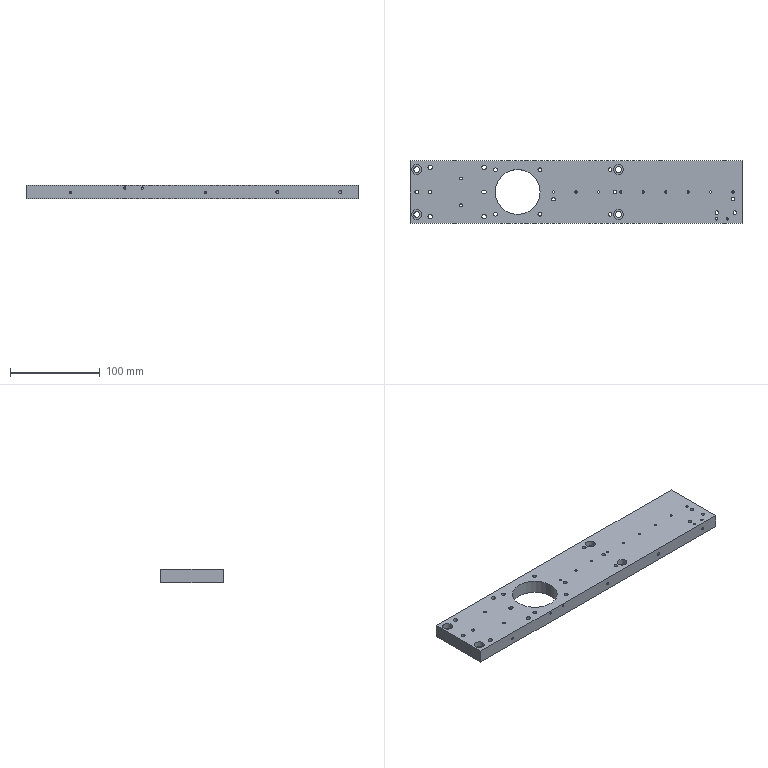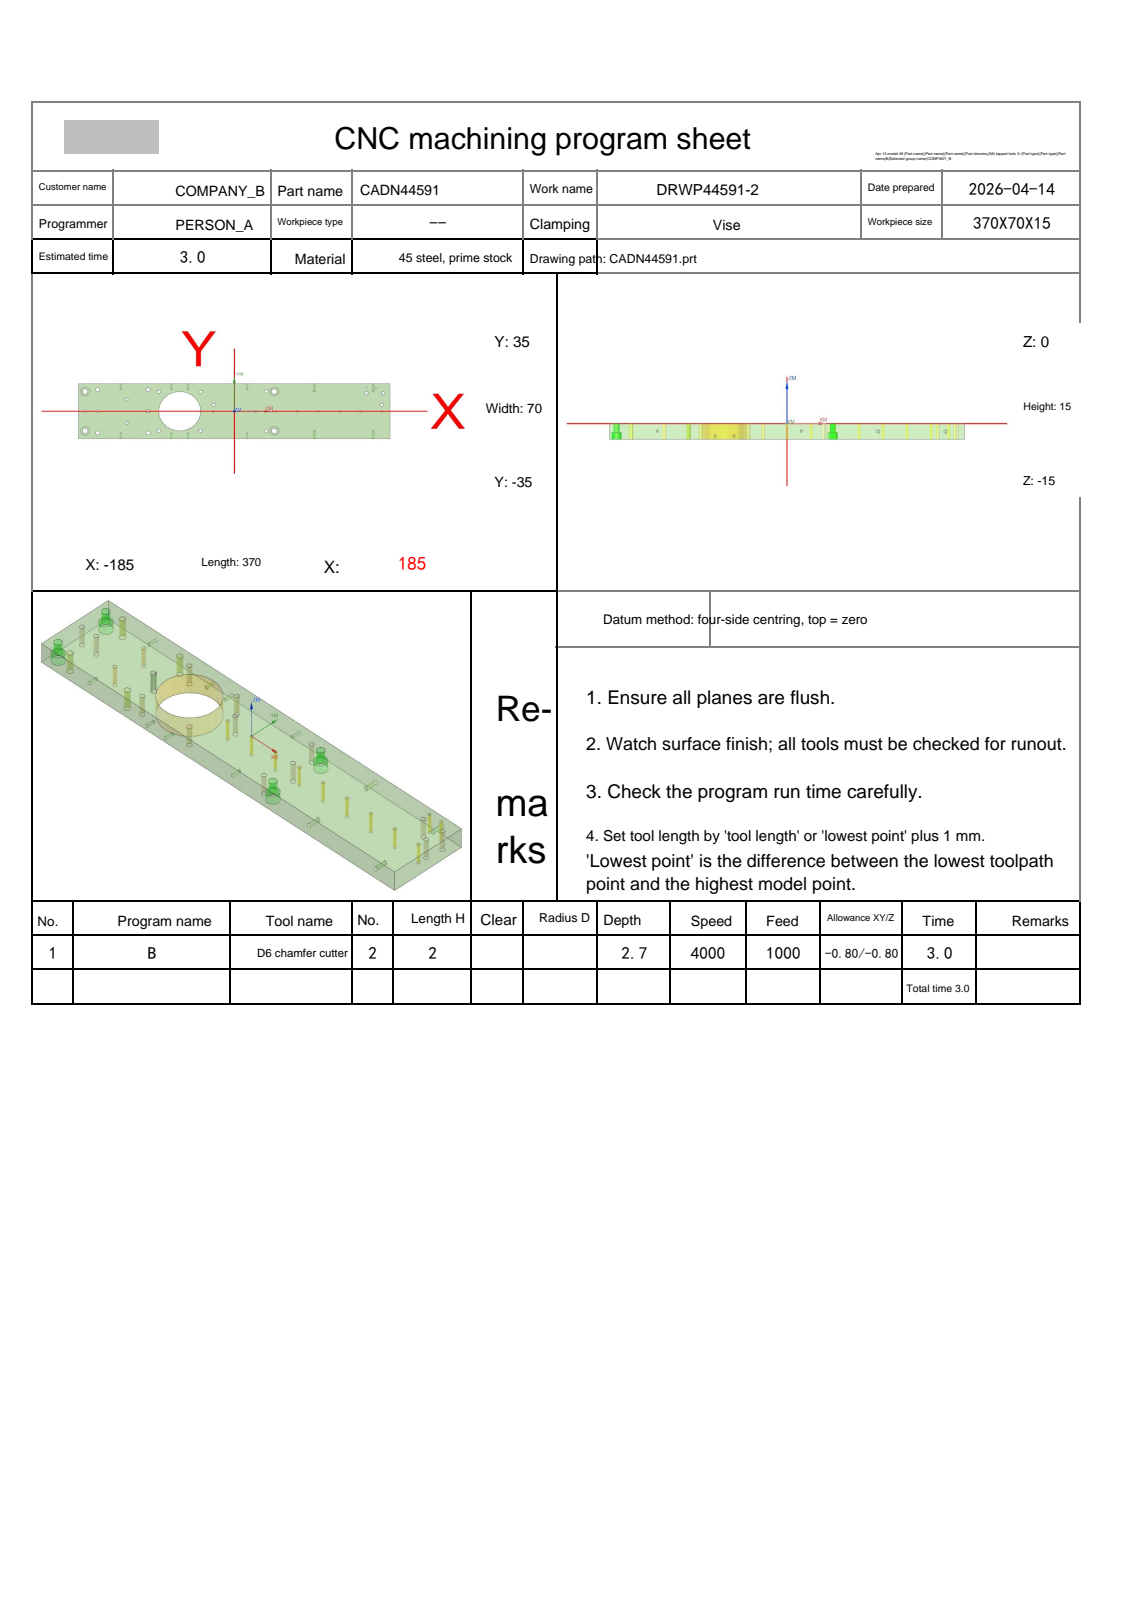NC program | NX | posted by the shop | part box 370 x 70 x 15 mm
Whole program:
%
O0001
(Machine time: 3.20 MIN)
(===Total Tool:1===)
(T2=D6 chamfer cutter   D=6.   R=0.   D-  H02 Z=-2.7  )
G80 G90 G17 G49 G40
G91 G28 Z0
M01
N1 T02 M06
(D6 chamfer cutter  D=6. R=0. H=02 ce=0.00 di=0.00)
G00 G90 G54 X156.5 Y30. M03 S2000
G43 H02 Z20.
M08
G98 G81 X156.5 Y30. Z-1.75 R3. F100.
X168.5
X175. Y0.0
X150.
X125.
X100.
X75.
X50.
X25.
X0.0
X-25.
G80
G00 Z20.
G00 G90 X-128. Y15. M03 S2000
Z20.
G98 G81 X-128. Y15. Z-2.2 R3. F100.
Y-15.
G80
G00 Z20.
G00 G90 X175. Y8. M03 S2000
Z20.
G98 G81 X175. Y8. Z-2.3 R3. F100.
X177. Y23.
X157.
X38. Y25.
X43.5 Y0.0
X38. Y-25.
X-25. Y8.
X-162.5 Y0.0
X-177.5
G80
G00 Z20.
G00 G90 X-40.251 Y-24.749 M03 S2000
Z20.
G98 G81 X-40.251 Y-24.749 Z-2.7 R3. F100.
Y24.749
X-89.749
Y-24.749
G80
G00 Z20.
G00 G90 X-102.593 Y28.194 M03 S4000
Z20.
Z-1.1
G01 Z-1.6 F300.
X-102.7 Y29.
G03 X-104.2 Y27.5 I0.0 J-1.5
X-102.5 Y25.8 I1.7 J0.0
X-100.8 Y27.5 I0.0 J1.7
X-102.5 Y29.2 I-1.7 J0.0
X-104.2 Y27.5 I0.0 J-1.7
X-102.7 Y26. I1.5 J0.0
G01 X-102.593 Y26.806
Z-1.1
G00 Z20.
Y-26.806
Z-1.1
G01 Z-1.6
X-102.7 Y-26.
G03 X-104.2 Y-27.5 I0.0 J-1.5
X-102.5 Y-29.2 I1.7 J0.0
X-100.8 Y-27.5 I0.0 J1.7
X-102.5 Y-25.8 I-1.7 J0.0
X-104.2 Y-27.5 I0.0 J-1.7
X-102.7 Y-29. I1.5 J0.0
G01 X-102.593 Y-28.194
Z-1.1
G00 Z20.
X-162.593 Y-26.806
Z-1.1
G01 Z-1.6
X-162.7 Y-26.
G03 X-164.2 Y-27.5 I0.0 J-1.5
X-162.5 Y-29.2 I1.7 J0.0
X-160.8 Y-27.5 I0.0 J1.7
X-162.5 Y-25.8 I-1.7 J0.0
X-164.2 Y-27.5 I0.0 J-1.7
X-162.7 Y-29. I1.5 J0.0
G01 X-162.593 Y-28.194
Z-1.1
G00 Z20.
Y28.194
Z-1.1
G01 Z-1.6
X-162.7 Y29.
G03 X-164.2 Y27.5 I0.0 J-1.5
X-162.5 Y25.8 I1.7 J0.0
X-160.8 Y27.5 I0.0 J1.7
X-162.5 Y29.2 I-1.7 J0.0
X-164.2 Y27.5 I0.0 J-1.7
X-162.7 Y26. I1.5 J0.0
G01 X-162.593 Y26.806
Z-1.1
G00 Z20.
G00 G90 X-177.816 Y25.949 M03 S4000
Z20.
Z-1.1
G01 Z-1.6 F600.
X-178. Y26.5
G03 X-179.5 Y25. I0.0 J-1.5
X-177.5 Y23. I2. J0.0
X-175.5 Y25. I0.0 J2.
X-177.5 Y27. I-2. J0.0
X-179.5 Y25. I0.0 J-2.
X-178. Y23.5 I1.5 J0.0
G01 X-177.816 Y24.051
Z-1.1
G00 Z20.
Y-24.051
Z-1.1
G01 Z-1.6
X-178. Y-23.5
G03 X-179.5 Y-25. I0.0 J-1.5
X-177.5 Y-27. I2. J0.0
X-175.5 Y-25. I0.0 J2.
X-177.5 Y-23. I-2. J0.0
X-179.5 Y-25. I0.0 J-2.
X-178. Y-26.5 I1.5 J0.0
G01 X-177.816 Y-25.949
Z-1.1
G00 Z20.
X47.184 Y-24.051
Z-1.1
G01 Z-1.6
X47. Y-23.5
G03 X45.5 Y-25. I0.0 J-1.5
X47.5 Y-27. I2. J0.0
X49.5 Y-25. I0.0 J2.
X47.5 Y-23. I-2. J0.0
X45.5 Y-25. I0.0 J-2.
X47. Y-26.5 I1.5 J0.0
G01 X47.184 Y-25.949
Z-1.1
G00 Z20.
Y25.949
Z-1.1
G01 Z-1.6
X47. Y26.5
G03 X45.5 Y25. I0.0 J-1.5
X47.5 Y23. I2. J0.0
X49.5 Y25. I0.0 J2.
X47.5 Y27. I-2. J0.0
X45.5 Y25. I0.0 J-2.
X47. Y23.5 I1.5 J0.0
G01 X47.184 Y24.051
Z-1.1
G00 Z20.
G00 G90 X-103.544 Y1.184 M03 S4000
Z20.
Z2.5
G01 X-103.742 Y1.071 Z2.417 F1000.
X-103.921 Y.921 Z2.332
X-104.071 Y.742 Z2.247
X-104.186 Y.539 Z2.162
X-104.263 Y.319 Z2.077
X-104.3 Y.088 Z1.992
Y-.088 Z1.928
X-104.263 Y-.319 Z1.843
X-104.186 Y-.539 Z1.758
X-104.071 Y-.742 Z1.673
X-103.921 Y-.921 Z1.588
X-103.742 Y-1.071 Z1.503
X-103.539 Y-1.186 Z1.418
X-103.319 Y-1.263 Z1.333
X-103.088 Y-1.3 Z1.248
X-101.912 Z.82
X-101.681 Y-1.263 Z.735
X-101.461 Y-1.186 Z.65
X-101.258 Y-1.071 Z.565
X-101.079 Y-.921 Z.48
X-100.929 Y-.742 Z.395
X-100.814 Y-.539 Z.31
X-100.737 Y-.319 Z.225
X-100.7 Y-.088 Z.14
Y.088 Z.076
X-100.737 Y.319 Z-.009
X-100.814 Y.539 Z-.094
X-100.929 Y.742 Z-.179
X-101.079 Y.921 Z-.264
X-101.258 Y1.071 Z-.349
X-101.461 Y1.186 Z-.434
X-101.681 Y1.263 Z-.519
X-101.912 Y1.3 Z-.604
X-103. Z-1.
G03 X-104.3 Y0.0 I0.0 J-1.3
X-103. Y-1.3 I1.3 J0.0
G01 X-102.
G03 X-100.7 Y0.0 I0.0 J1.3
X-102. Y1.3 I-1.3 J0.0
G01 X-103.
G03 X-103.488 Y1.205 I0.0 J-1.3
G01 Z1.5
G00 Z20.
X-42.58 Y-9.366
Z2.5
G01 X-42.314 Y-8.717 Z2.245
X-41.953 Y-7.713 Z1.857
X-41.637 Y-6.695 Z1.468
X-41.366 Y-5.663 Z1.08
X-41.14 Y-4.62 Z.692
X-40.961 Y-3.569 Z.304
X-40.827 Y-2.511 Z-.085
X-40.74 Y-1.448 Z-.473
X-40.7 Y-.382 Z-.861
Y0.0 Z-1.
G03 X-65. Y24.3 I-24.3 J0.0
X-89.3 Y0.0 I0.0 J-24.3
X-65. Y-24.3 I24.3 J0.0
X-40.7 Y0.0 I0.0 J24.3
X-40.705 Y.5 I-24.3 J0.0
G01 Z1.5
G00 Z20.
X-185.7 Y26.657
Z2.5
G01 Y34.778 Z-.456
X-185.664 Y34.977 Z-.529
X-185.589 Y35.165 Z-.603
X-185.477 Y35.334 Z-.677
X-185.334 Y35.477 Z-.751
X-185.165 Y35.589 Z-.824
X-184.977 Y35.664 Z-.898
X-184.778 Y35.7 Z-.972
X-184.7 Z-1.
X184.7
G02 X185.7 Y34.7 I0.0 J-1.
G01 Y-34.7
G02 X184.7 Y-35.7 I-1. J0.0
G01 X-184.7
G02 X-185.7 Y-34.7 I0.0 J1.
G01 Y34.7
G02 X-184.7 Y35.7 I1. J0.0
G01 X-184.2
Z1.5
G00 Z20.
M05
M09
G91 G28 Z0.0
G91 G28 Y0.0
M30
%